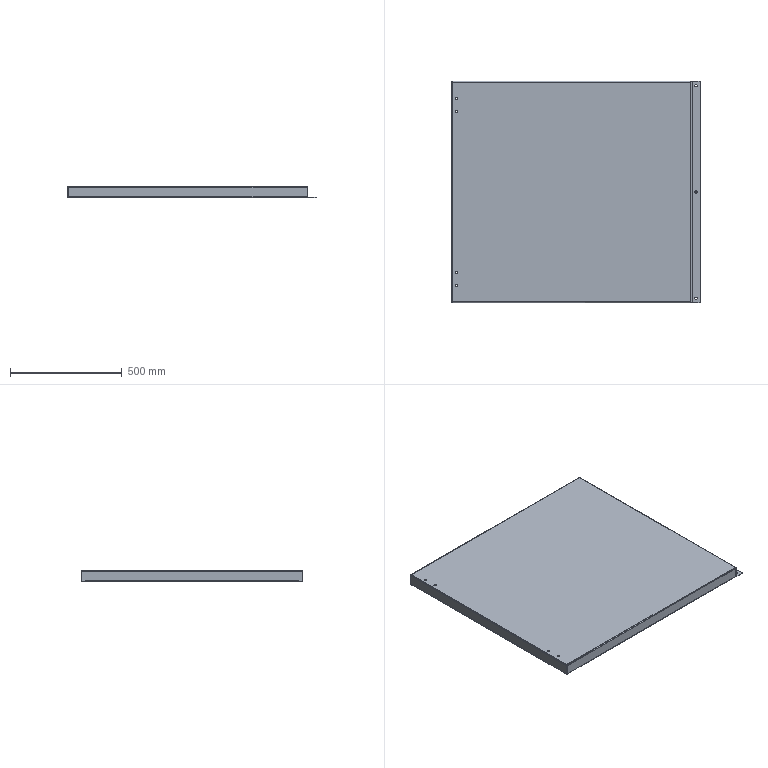Part | STEP file | B_SYL0380DJ1008_2_9_1-1_STEP | 1 solid | 98 faces | box 1114 x 994 x 52 mm | volume 2704262 mm3 | plane 58 | cylinder 32 | spline 8 | commonest cylinder face diameters 4 x8 8 x8 10.5 x8 11 x6 10 x2